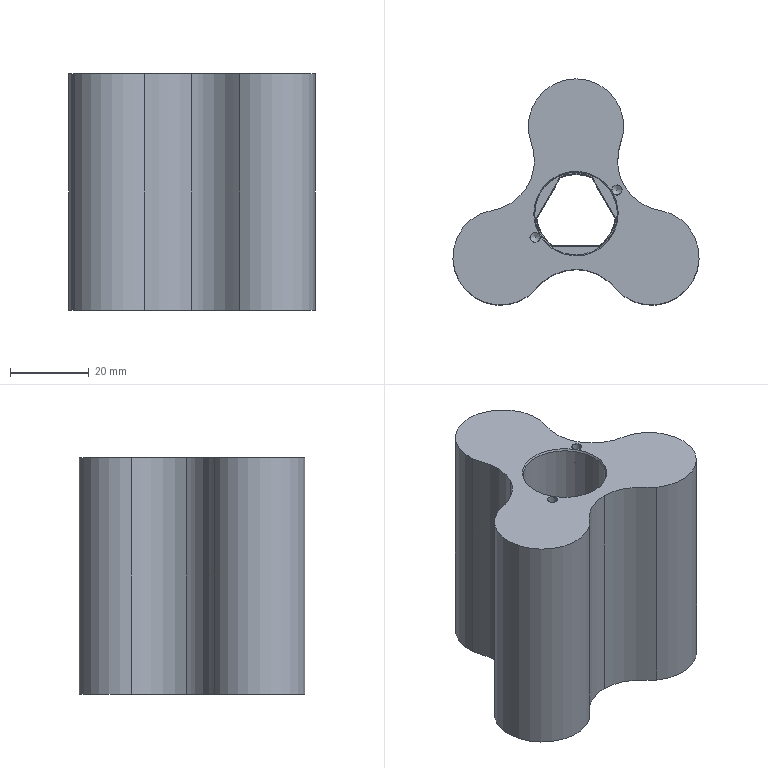Part | 1 solid | 50 faces | box 62.563 x 57.43 x 60 mm | volume 98387 mm3 | cone 18 | plane 13 | cylinder 13 | spline 6 | commonest cylinder face diameters 4.2 x3 20 x3 24.253 x3 2.5 x2 21 x1 24 x1
STEP:
#1=CARTESIAN_POINT('',(0.,-14.155,0.));
#2=VERTEX_POINT('',#1);
#3=CARTESIAN_POINT('',(-12.154,-20.96,0.));
#4=VERTEX_POINT('',#3);
#5=CARTESIAN_POINT('',(0.,-14.155,0.));
#6=CARTESIAN_POINT('',(-1.208,-14.163,0.));
#7=CARTESIAN_POINT('',(-3.582,-14.493,0.));
#8=CARTESIAN_POINT('',(-6.901,-15.987,0.));
#9=CARTESIAN_POINT('',(-9.683,-18.323,0.));
#10=CARTESIAN_POINT('',(-11.16,-20.256,0.));
#11=CARTESIAN_POINT('',(-12.154,-20.96,0.));
#12=B_SPLINE_CURVE_WITH_KNOTS('',3,(#5,#6,#7,#8,#9,#10,#11),.UNSPECIFIED.,.F.,.F.,(4,1,1,1,4),(0.,0.003576,0.007152,0.01073,0.0143),.UNSPECIFIED.);
#13=EDGE_CURVE('',#2,#4,#12,.T.);
#14=ORIENTED_EDGE('',*,*,#13,.F.);
#15=CARTESIAN_POINT('',(12.154,-20.96,0.));
#16=VERTEX_POINT('',#15);
#17=CARTESIAN_POINT('',(12.154,-20.96,0.));
#18=CARTESIAN_POINT('',(11.156,-20.253,0.));
#19=CARTESIAN_POINT('',(9.676,-18.315,0.));
#20=CARTESIAN_POINT('',(6.903,-15.991,0.));
#21=CARTESIAN_POINT('',(3.605,-14.498,0.));
#22=CARTESIAN_POINT('',(1.208,-14.163,0.));
#23=CARTESIAN_POINT('',(0.,-14.155,0.));
#24=B_SPLINE_CURVE_WITH_KNOTS('',3,(#17,#18,#19,#20,#21,#22,#23),.UNSPECIFIED.,.F.,.F.,(4,1,1,1,4),(0.,0.003619,0.007238,0.01086,0.01448),.UNSPECIFIED.);
#25=EDGE_CURVE('',#16,#2,#24,.T.);
#26=ORIENTED_EDGE('',*,*,#25,.F.);
#27=CARTESIAN_POINT('',(24.229,-0.04541,0.));
#28=VERTEX_POINT('',#27);
#29=CARTESIAN_POINT('',(19.155,-11.059,0.));
#30=DIRECTION('',(0.,0.,-1.));
#31=DIRECTION('',(-0.866,-0.5,0.));
#32=AXIS2_PLACEMENT_3D('',#29,#30,#31);
#33=CIRCLE('',#32,12.126);
#34=EDGE_CURVE('',#28,#16,#33,.T.);
#35=ORIENTED_EDGE('',*,*,#34,.F.);
#36=CARTESIAN_POINT('',(12.259,7.078,0.));
#37=VERTEX_POINT('',#36);
#38=CARTESIAN_POINT('',(12.259,7.078,0.));
#39=CARTESIAN_POINT('',(12.87,6.035,0.));
#40=CARTESIAN_POINT('',(14.342,4.144,0.));
#41=CARTESIAN_POINT('',(17.296,2.017,0.));
#42=CARTESIAN_POINT('',(20.71,0.7759,0.));
#43=CARTESIAN_POINT('',(23.122,0.4633,0.));
#44=CARTESIAN_POINT('',(24.229,-0.04541,0.));
#45=B_SPLINE_CURVE_WITH_KNOTS('',3,(#38,#39,#40,#41,#42,#43,#44),.UNSPECIFIED.,.F.,.F.,(4,1,1,1,4),(0.,0.003576,0.007152,0.01073,0.0143),.UNSPECIFIED.);
#46=EDGE_CURVE('',#37,#28,#45,.T.);
#47=ORIENTED_EDGE('',*,*,#46,.F.);
#48=CARTESIAN_POINT('',(12.075,21.006,0.));
#49=VERTEX_POINT('',#48);
#50=CARTESIAN_POINT('',(12.075,21.006,0.));
#51=CARTESIAN_POINT('',(11.962,19.788,0.));
#52=CARTESIAN_POINT('',(11.023,17.537,0.));
#53=CARTESIAN_POINT('',(10.398,13.974,0.));
#54=CARTESIAN_POINT('',(10.753,10.371,0.));
#55=CARTESIAN_POINT('',(11.662,8.128,0.));
#56=CARTESIAN_POINT('',(12.259,7.078,0.));
#57=B_SPLINE_CURVE_WITH_KNOTS('',3,(#50,#51,#52,#53,#54,#55,#56),.UNSPECIFIED.,.F.,.F.,(4,1,1,1,4),(0.,0.003619,0.007238,0.01086,0.01448),.UNSPECIFIED.);
#58=EDGE_CURVE('',#49,#37,#57,.T.);
#59=ORIENTED_EDGE('',*,*,#58,.F.);
#60=CARTESIAN_POINT('',(-12.075,21.006,0.));
#61=VERTEX_POINT('',#60);
#62=CARTESIAN_POINT('',(0.,22.118,0.));
#63=DIRECTION('',(0.,0.,-1.));
#64=DIRECTION('',(-0.866,-0.5,0.));
#65=AXIS2_PLACEMENT_3D('',#62,#63,#64);
#66=CIRCLE('',#65,12.126);
#67=EDGE_CURVE('',#61,#49,#66,.T.);
#68=ORIENTED_EDGE('',*,*,#67,.F.);
#69=CARTESIAN_POINT('',(-12.259,7.078,0.));
#70=VERTEX_POINT('',#69);
#71=CARTESIAN_POINT('',(-12.259,7.078,0.));
#72=CARTESIAN_POINT('',(-11.662,8.128,0.));
#73=CARTESIAN_POINT('',(-10.76,10.348,0.));
#74=CARTESIAN_POINT('',(-10.395,13.97,0.));
#75=CARTESIAN_POINT('',(-11.027,17.548,0.));
#76=CARTESIAN_POINT('',(-11.962,19.793,0.));
#77=CARTESIAN_POINT('',(-12.075,21.006,0.));
#78=B_SPLINE_CURVE_WITH_KNOTS('',3,(#71,#72,#73,#74,#75,#76,#77),.UNSPECIFIED.,.F.,.F.,(4,1,1,1,4),(0.,0.003576,0.007152,0.01073,0.0143),.UNSPECIFIED.);
#79=EDGE_CURVE('',#70,#61,#78,.T.);
#80=ORIENTED_EDGE('',*,*,#79,.F.);
#81=CARTESIAN_POINT('',(-24.229,-0.04543,0.));
#82=VERTEX_POINT('',#81);
#83=CARTESIAN_POINT('',(-24.229,-0.04543,0.));
#84=CARTESIAN_POINT('',(-23.118,0.4655,0.));
#85=CARTESIAN_POINT('',(-20.699,0.7776,0.));
#86=CARTESIAN_POINT('',(-17.3,2.018,0.));
#87=CARTESIAN_POINT('',(-14.358,4.127,0.));
#88=CARTESIAN_POINT('',(-12.87,6.036,0.));
#89=CARTESIAN_POINT('',(-12.259,7.078,0.));
#90=B_SPLINE_CURVE_WITH_KNOTS('',3,(#83,#84,#85,#86,#87,#88,#89),.UNSPECIFIED.,.F.,.F.,(4,1,1,1,4),(0.,0.003619,0.007238,0.01086,0.01448),.UNSPECIFIED.);
#91=EDGE_CURVE('',#82,#70,#90,.T.);
#92=ORIENTED_EDGE('',*,*,#91,.F.);
#93=CARTESIAN_POINT('',(-19.155,-11.059,0.));
#94=DIRECTION('',(0.,0.,-1.));
#95=DIRECTION('',(-0.866,-0.5,0.));
#96=AXIS2_PLACEMENT_3D('',#93,#94,#95);
#97=CIRCLE('',#96,12.126);
#98=EDGE_CURVE('',#4,#82,#97,.T.);
#99=ORIENTED_EDGE('',*,*,#98,.F.);
#100=EDGE_LOOP('',(#14,#26,#35,#47,#59,#68,#80,#92,#99));
#101=FACE_BOUND('',#100,.T.);
#102=CARTESIAN_POINT('',(-9.43,-5.126,0.));
#103=VERTEX_POINT('',#102);
#104=CARTESIAN_POINT('',(-9.154,-5.604,0.));
#105=VERTEX_POINT('',#104);
#106=CARTESIAN_POINT('',(-10.392,-6.,0.));
#107=DIRECTION('',(0.,0.,1.));
#108=DIRECTION('',(0.866,0.5,0.));
#109=AXIS2_PLACEMENT_3D('',#106,#107,#108);
#110=CIRCLE('',#109,1.3);
#111=EDGE_CURVE('',#103,#105,#110,.T.);
#112=ORIENTED_EDGE('',*,*,#111,.F.);
#113=CARTESIAN_POINT('',(9.154,5.604,0.));
#114=VERTEX_POINT('',#113);
#115=CARTESIAN_POINT('',(0.,0.,0.));
#116=DIRECTION('',(0.,0.,-1.));
#117=DIRECTION('',(-0.866,-0.5,0.));
#118=AXIS2_PLACEMENT_3D('',#115,#116,#117);
#119=CIRCLE('',#118,10.733);
#120=EDGE_CURVE('',#103,#114,#119,.T.);
#121=ORIENTED_EDGE('',*,*,#120,.T.);
#122=CARTESIAN_POINT('',(9.43,5.126,0.));
#123=VERTEX_POINT('',#122);
#124=CARTESIAN_POINT('',(10.392,6.,0.));
#125=DIRECTION('',(0.,0.,1.));
#126=DIRECTION('',(0.866,0.5,0.));
#127=AXIS2_PLACEMENT_3D('',#124,#125,#126);
#128=CIRCLE('',#127,1.3);
#129=EDGE_CURVE('',#123,#114,#128,.T.);
#130=ORIENTED_EDGE('',*,*,#129,.F.);
#131=CARTESIAN_POINT('',(0.,0.,0.));
#132=DIRECTION('',(0.,0.,-1.));
#133=DIRECTION('',(-0.866,-0.5,0.));
#134=AXIS2_PLACEMENT_3D('',#131,#132,#133);
#135=CIRCLE('',#134,10.733);
#136=EDGE_CURVE('',#123,#105,#135,.T.);
#137=ORIENTED_EDGE('',*,*,#136,.T.);
#138=EDGE_LOOP('',(#112,#121,#130,#137));
#139=FACE_BOUND('',#138,.T.);
#140=CARTESIAN_POINT('',(-6.815,-16.188,0.));
#141=DIRECTION('',(0.,0.,-1.));
#142=DIRECTION('',(-0.866,-0.5,0.));
#143=AXIS2_PLACEMENT_3D('',#140,#141,#142);
#144=PLANE('',#143);
#145=ADVANCED_FACE('',(#101,#139),#144,.F.);
#146=CARTESIAN_POINT('',(3.928,9.196,-50.3));
#147=VERTEX_POINT('',#146);
#148=CARTESIAN_POINT('',(3.928,9.196,-15.4));
#149=VERTEX_POINT('',#148);
#150=CARTESIAN_POINT('',(3.928,9.196,-60.));
#151=DIRECTION('',(0.,0.,1.));
#152=VECTOR('',#151,1000.);
#153=LINE('',#150,#152);
#154=EDGE_CURVE('',#147,#149,#153,.T.);
#155=ORIENTED_EDGE('',*,*,#154,.T.);
#156=CARTESIAN_POINT('',(-3.928,9.196,-15.4));
#157=VERTEX_POINT('',#156);
#158=CARTESIAN_POINT('',(0.,0.,-15.4));
#159=DIRECTION('',(0.,0.,1.));
#160=DIRECTION('',(0.866,0.5,0.));
#161=AXIS2_PLACEMENT_3D('',#158,#159,#160);
#162=CIRCLE('',#161,10.);
#163=EDGE_CURVE('',#149,#157,#162,.T.);
#164=ORIENTED_EDGE('',*,*,#163,.T.);
#165=CARTESIAN_POINT('',(-3.928,9.196,-50.3));
#166=VERTEX_POINT('',#165);
#167=CARTESIAN_POINT('',(-3.928,9.196,-60.));
#168=DIRECTION('',(0.,0.,1.));
#169=VECTOR('',#168,1000.);
#170=LINE('',#167,#169);
#171=EDGE_CURVE('',#166,#157,#170,.T.);
#172=ORIENTED_EDGE('',*,*,#171,.F.);
#173=CARTESIAN_POINT('',(0.,0.,-50.3));
#174=DIRECTION('',(0.,0.,-1.));
#175=DIRECTION('',(-0.866,-0.5,0.));
#176=AXIS2_PLACEMENT_3D('',#173,#174,#175);
#177=CIRCLE('',#176,10.);
#178=EDGE_CURVE('',#166,#147,#177,.T.);
#179=ORIENTED_EDGE('',*,*,#178,.T.);
#180=EDGE_LOOP('',(#155,#164,#172,#179));
#181=FACE_BOUND('',#180,.T.);
#182=CARTESIAN_POINT('',(0.,0.,-60.));
#183=DIRECTION('',(0.,0.,1.));
#184=DIRECTION('',(0.866,0.5,0.));
#185=AXIS2_PLACEMENT_3D('',#182,#183,#184);
#186=CYLINDRICAL_SURFACE('',#185,10.);
#187=ADVANCED_FACE('',(#181),#186,.F.);
#188=CARTESIAN_POINT('',(9.928,-1.196,-50.3));
#189=VERTEX_POINT('',#188);
#190=CARTESIAN_POINT('',(9.928,-1.196,-15.4));
#191=VERTEX_POINT('',#190);
#192=CARTESIAN_POINT('',(9.928,-1.196,-60.));
#193=DIRECTION('',(0.,0.,1.));
#194=VECTOR('',#193,1000.);
#195=LINE('',#192,#194);
#196=EDGE_CURVE('',#189,#191,#195,.T.);
#197=ORIENTED_EDGE('',*,*,#196,.T.);
#198=CARTESIAN_POINT('',(3.928,9.196,-15.4));
#199=DIRECTION('',(-0.5,0.866,0.));
#200=VECTOR('',#199,1000.);
#201=LINE('',#198,#200);
#202=EDGE_CURVE('',#191,#149,#201,.T.);
#203=ORIENTED_EDGE('',*,*,#202,.T.);
#204=ORIENTED_EDGE('',*,*,#154,.F.);
#205=CARTESIAN_POINT('',(9.928,-1.196,-50.3));
#206=DIRECTION('',(0.5,-0.866,0.));
#207=VECTOR('',#206,1000.);
#208=LINE('',#205,#207);
#209=EDGE_CURVE('',#147,#189,#208,.T.);
#210=ORIENTED_EDGE('',*,*,#209,.T.);
#211=EDGE_LOOP('',(#197,#203,#204,#210));
#212=FACE_BOUND('',#211,.T.);
#213=CARTESIAN_POINT('',(3.928,9.196,-60.));
#214=DIRECTION('',(0.866,0.5,0.));
#215=DIRECTION('',(0.,0.,-1.));
#216=AXIS2_PLACEMENT_3D('',#213,#214,#215);
#217=PLANE('',#216);
#218=ADVANCED_FACE('',(#212),#217,.F.);
#219=CARTESIAN_POINT('',(6.,-8.,-50.3));
#220=VERTEX_POINT('',#219);
#221=CARTESIAN_POINT('',(6.,-8.,-15.4));
#222=VERTEX_POINT('',#221);
#223=CARTESIAN_POINT('',(6.,-8.,-60.));
#224=DIRECTION('',(0.,0.,1.));
#225=VECTOR('',#224,1000.);
#226=LINE('',#223,#225);
#227=EDGE_CURVE('',#220,#222,#226,.T.);
#228=ORIENTED_EDGE('',*,*,#227,.T.);
#229=CARTESIAN_POINT('',(0.,0.,-15.4));
#230=DIRECTION('',(0.,0.,1.));
#231=DIRECTION('',(0.866,0.5,0.));
#232=AXIS2_PLACEMENT_3D('',#229,#230,#231);
#233=CIRCLE('',#232,10.);
#234=EDGE_CURVE('',#222,#191,#233,.T.);
#235=ORIENTED_EDGE('',*,*,#234,.T.);
#236=ORIENTED_EDGE('',*,*,#196,.F.);
#237=CARTESIAN_POINT('',(0.,0.,-50.3));
#238=DIRECTION('',(0.,0.,-1.));
#239=DIRECTION('',(-0.866,-0.5,0.));
#240=AXIS2_PLACEMENT_3D('',#237,#238,#239);
#241=CIRCLE('',#240,10.);
#242=EDGE_CURVE('',#189,#220,#241,.T.);
#243=ORIENTED_EDGE('',*,*,#242,.T.);
#244=EDGE_LOOP('',(#228,#235,#236,#243));
#245=FACE_BOUND('',#244,.T.);
#246=CARTESIAN_POINT('',(0.,0.,-60.));
#247=DIRECTION('',(0.,0.,1.));
#248=DIRECTION('',(0.866,0.5,0.));
#249=AXIS2_PLACEMENT_3D('',#246,#247,#248);
#250=CYLINDRICAL_SURFACE('',#249,10.);
#251=ADVANCED_FACE('',(#245),#250,.F.);
#252=CARTESIAN_POINT('',(-6.,-8.,-50.3));
#253=VERTEX_POINT('',#252);
#254=CARTESIAN_POINT('',(-6.,-8.,-15.4));
#255=VERTEX_POINT('',#254);
#256=CARTESIAN_POINT('',(-6.,-8.,-60.));
#257=DIRECTION('',(0.,0.,1.));
#258=VECTOR('',#257,1000.);
#259=LINE('',#256,#258);
#260=EDGE_CURVE('',#253,#255,#259,.T.);
#261=ORIENTED_EDGE('',*,*,#260,.T.);
#262=CARTESIAN_POINT('',(6.,-8.,-15.4));
#263=DIRECTION('',(1.,0.,0.));
#264=VECTOR('',#263,1000.);
#265=LINE('',#262,#264);
#266=EDGE_CURVE('',#255,#222,#265,.T.);
#267=ORIENTED_EDGE('',*,*,#266,.T.);
#268=ORIENTED_EDGE('',*,*,#227,.F.);
#269=CARTESIAN_POINT('',(-6.,-8.,-50.3));
#270=DIRECTION('',(-1.,0.,0.));
#271=VECTOR('',#270,1000.);
#272=LINE('',#269,#271);
#273=EDGE_CURVE('',#220,#253,#272,.T.);
#274=ORIENTED_EDGE('',*,*,#273,.T.);
#275=EDGE_LOOP('',(#261,#267,#268,#274));
#276=FACE_BOUND('',#275,.T.);
#277=CARTESIAN_POINT('',(6.,-8.,-60.));
#278=DIRECTION('',(0.,-1.,0.));
#279=DIRECTION('',(-1.,0.,0.));
#280=AXIS2_PLACEMENT_3D('',#277,#278,#279);
#281=PLANE('',#280);
#282=ADVANCED_FACE('',(#276),#281,.F.);
#283=CARTESIAN_POINT('',(-9.928,-1.196,-50.3));
#284=VERTEX_POINT('',#283);
#285=CARTESIAN_POINT('',(-9.928,-1.196,-15.4));
#286=VERTEX_POINT('',#285);
#287=CARTESIAN_POINT('',(-9.928,-1.196,-60.));
#288=DIRECTION('',(0.,0.,1.));
#289=VECTOR('',#288,1000.);
#290=LINE('',#287,#289);
#291=EDGE_CURVE('',#284,#286,#290,.T.);
#292=ORIENTED_EDGE('',*,*,#291,.T.);
#293=CARTESIAN_POINT('',(0.,0.,-15.4));
#294=DIRECTION('',(0.,0.,1.));
#295=DIRECTION('',(0.866,0.5,0.));
#296=AXIS2_PLACEMENT_3D('',#293,#294,#295);
#297=CIRCLE('',#296,10.);
#298=EDGE_CURVE('',#286,#255,#297,.T.);
#299=ORIENTED_EDGE('',*,*,#298,.T.);
#300=ORIENTED_EDGE('',*,*,#260,.F.);
#301=CARTESIAN_POINT('',(0.,0.,-50.3));
#302=DIRECTION('',(0.,0.,-1.));
#303=DIRECTION('',(-0.866,-0.5,0.));
#304=AXIS2_PLACEMENT_3D('',#301,#302,#303);
#305=CIRCLE('',#304,10.);
#306=EDGE_CURVE('',#253,#284,#305,.T.);
#307=ORIENTED_EDGE('',*,*,#306,.T.);
#308=EDGE_LOOP('',(#292,#299,#300,#307));
#309=FACE_BOUND('',#308,.T.);
#310=CARTESIAN_POINT('',(0.,0.,-60.));
#311=DIRECTION('',(0.,0.,1.));
#312=DIRECTION('',(0.866,0.5,0.));
#313=AXIS2_PLACEMENT_3D('',#310,#311,#312);
#314=CYLINDRICAL_SURFACE('',#313,10.);
#315=ADVANCED_FACE('',(#309),#314,.F.);
#316=ORIENTED_EDGE('',*,*,#171,.T.);
#317=CARTESIAN_POINT('',(-9.928,-1.196,-15.4));
#318=DIRECTION('',(-0.5,-0.866,0.));
#319=VECTOR('',#318,1000.);
#320=LINE('',#317,#319);
#321=EDGE_CURVE('',#157,#286,#320,.T.);
#322=ORIENTED_EDGE('',*,*,#321,.T.);
#323=ORIENTED_EDGE('',*,*,#291,.F.);
#324=CARTESIAN_POINT('',(-3.928,9.196,-50.3));
#325=DIRECTION('',(0.5,0.866,0.));
#326=VECTOR('',#325,1000.);
#327=LINE('',#324,#326);
#328=EDGE_CURVE('',#284,#166,#327,.T.);
#329=ORIENTED_EDGE('',*,*,#328,.T.);
#330=EDGE_LOOP('',(#316,#322,#323,#329));
#331=FACE_BOUND('',#330,.T.);
#332=CARTESIAN_POINT('',(-9.928,-1.196,-60.));
#333=DIRECTION('',(-0.866,0.5,0.));
#334=DIRECTION('',(0.5,0.866,0.));
#335=AXIS2_PLACEMENT_3D('',#332,#333,#334);
#336=PLANE('',#335);
#337=ADVANCED_FACE('',(#331),#336,.F.);
#338=ORIENTED_EDGE('',*,*,#13,.T.);
#339=CARTESIAN_POINT('',(-12.154,-20.96,-60.));
#340=VERTEX_POINT('',#339);
#341=CARTESIAN_POINT('',(-12.154,-20.96,-60.));
#342=DIRECTION('',(0.,0.,1.));
#343=VECTOR('',#342,1000.);
#344=LINE('',#341,#343);
#345=EDGE_CURVE('',#340,#4,#344,.T.);
#346=ORIENTED_EDGE('',*,*,#345,.F.);
#347=CARTESIAN_POINT('',(0.,-14.155,-60.));
#348=VERTEX_POINT('',#347);
#349=CARTESIAN_POINT('',(0.,-14.155,-60.));
#350=CARTESIAN_POINT('',(-1.208,-14.163,-60.));
#351=CARTESIAN_POINT('',(-3.582,-14.493,-60.));
#352=CARTESIAN_POINT('',(-6.901,-15.987,-60.));
#353=CARTESIAN_POINT('',(-9.683,-18.323,-60.));
#354=CARTESIAN_POINT('',(-11.16,-20.256,-60.));
#355=CARTESIAN_POINT('',(-12.154,-20.96,-60.));
#356=B_SPLINE_CURVE_WITH_KNOTS('',3,(#349,#350,#351,#352,#353,#354,#355),.UNSPECIFIED.,.F.,.F.,(4,1,1,1,4),(0.,0.003576,0.007152,0.01073,0.0143),.UNSPECIFIED.);
#357=EDGE_CURVE('',#348,#340,#356,.T.);
#358=ORIENTED_EDGE('',*,*,#357,.F.);
#359=CARTESIAN_POINT('',(0.,-14.155,-60.));
#360=DIRECTION('',(0.,0.,1.));
#361=VECTOR('',#360,1000.);
#362=LINE('',#359,#361);
#363=EDGE_CURVE('',#348,#2,#362,.T.);
#364=ORIENTED_EDGE('',*,*,#363,.T.);
#365=EDGE_LOOP('',(#338,#346,#358,#364));
#366=FACE_BOUND('',#365,.T.);
#367=CARTESIAN_POINT('',(0.,-14.155,-60.));
#368=CARTESIAN_POINT('',(0.,-14.155,0.));
#369=CARTESIAN_POINT('',(-1.199,-14.163,-60.));
#370=CARTESIAN_POINT('',(-1.199,-14.163,0.));
#371=CARTESIAN_POINT('',(-3.611,-14.497,-60.));
#372=CARTESIAN_POINT('',(-3.611,-14.497,0.));
#373=CARTESIAN_POINT('',(-6.932,-16.006,-60.));
#374=CARTESIAN_POINT('',(-6.932,-16.006,0.));
#375=CARTESIAN_POINT('',(-9.709,-18.356,-60.));
#376=CARTESIAN_POINT('',(-9.709,-18.356,0.));
#377=CARTESIAN_POINT('',(-11.176,-20.267,-60.));
#378=CARTESIAN_POINT('',(-11.176,-20.267,0.));
#379=CARTESIAN_POINT('',(-12.154,-20.96,-60.));
#380=CARTESIAN_POINT('',(-12.154,-20.96,0.));
#381=B_SPLINE_SURFACE_WITH_KNOTS('',3,1,((#367,#368),(#369,#370),(#371,#372),(#373,#374),(#375,#376),(#377,#378),(#379,#380)),.SURF_OF_LINEAR_EXTRUSION.,.F.,.F.,.F.,(4,1,1,1,4),(2,2),(-0.00002345,0.25,0.5,0.75,1.),(0.,1.),.UNSPECIFIED.);
#382=ADVANCED_FACE('',(#366),#381,.F.);
#383=ORIENTED_EDGE('',*,*,#98,.T.);
#384=CARTESIAN_POINT('',(-24.229,-0.04543,-60.));
#385=VERTEX_POINT('',#384);
#386=CARTESIAN_POINT('',(-24.229,-0.04543,-60.));
#387=DIRECTION('',(0.,0.,1.));
#388=VECTOR('',#387,1000.);
#389=LINE('',#386,#388);
#390=EDGE_CURVE('',#385,#82,#389,.T.);
#391=ORIENTED_EDGE('',*,*,#390,.F.);
#392=CARTESIAN_POINT('',(-19.155,-11.059,-60.));
#393=DIRECTION('',(0.,0.,-1.));
#394=DIRECTION('',(-0.866,-0.5,0.));
#395=AXIS2_PLACEMENT_3D('',#392,#393,#394);
#396=CIRCLE('',#395,12.126);
#397=EDGE_CURVE('',#340,#385,#396,.T.);
#398=ORIENTED_EDGE('',*,*,#397,.F.);
#399=ORIENTED_EDGE('',*,*,#345,.T.);
#400=EDGE_LOOP('',(#383,#391,#398,#399));
#401=FACE_BOUND('',#400,.T.);
#402=CARTESIAN_POINT('',(-19.155,-11.059,-60.));
#403=DIRECTION('',(0.,0.,1.));
#404=DIRECTION('',(0.866,0.5,0.));
#405=AXIS2_PLACEMENT_3D('',#402,#403,#404);
#406=CYLINDRICAL_SURFACE('',#405,12.126);
#407=ADVANCED_FACE('',(#401),#406,.T.);
#408=ORIENTED_EDGE('',*,*,#91,.T.);
#409=CARTESIAN_POINT('',(-12.259,7.078,-60.));
#410=VERTEX_POINT('',#409);
#411=CARTESIAN_POINT('',(-12.259,7.078,-60.));
#412=DIRECTION('',(0.,0.,1.));
#413=VECTOR('',#412,1000.);
#414=LINE('',#411,#413);
#415=EDGE_CURVE('',#410,#70,#414,.T.);
#416=ORIENTED_EDGE('',*,*,#415,.F.);
#417=CARTESIAN_POINT('',(-24.229,-0.04543,-60.));
#418=CARTESIAN_POINT('',(-23.118,0.4655,-60.));
#419=CARTESIAN_POINT('',(-20.699,0.7776,-60.));
#420=CARTESIAN_POINT('',(-17.3,2.018,-60.));
#421=CARTESIAN_POINT('',(-14.358,4.127,-60.));
#422=CARTESIAN_POINT('',(-12.87,6.036,-60.));
#423=CARTESIAN_POINT('',(-12.259,7.078,-60.));
#424=B_SPLINE_CURVE_WITH_KNOTS('',3,(#417,#418,#419,#420,#421,#422,#423),.UNSPECIFIED.,.F.,.F.,(4,1,1,1,4),(0.,0.003619,0.007238,0.01086,0.01448),.UNSPECIFIED.);
#425=EDGE_CURVE('',#385,#410,#424,.T.);
#426=ORIENTED_EDGE('',*,*,#425,.F.);
#427=ORIENTED_EDGE('',*,*,#390,.T.);
#428=EDGE_LOOP('',(#408,#416,#426,#427));
#429=FACE_BOUND('',#428,.T.);
#430=CARTESIAN_POINT('',(-24.229,-0.04543,-60.));
#431=CARTESIAN_POINT('',(-24.229,-0.04543,0.));
#432=CARTESIAN_POINT('',(-23.14,0.4552,-60.));
#433=CARTESIAN_POINT('',(-23.14,0.4552,0.));
#434=CARTESIAN_POINT('',(-20.752,0.7702,-60.));
#435=CARTESIAN_POINT('',(-20.752,0.7702,0.));
#436=CARTESIAN_POINT('',(-17.327,2.,-60.));
#437=CARTESIAN_POINT('',(-17.327,2.,0.));
#438=CARTESIAN_POINT('',(-14.361,4.121,-60.));
#439=CARTESIAN_POINT('',(-14.361,4.121,0.));
#440=CARTESIAN_POINT('',(-12.865,6.044,-60.));
#441=CARTESIAN_POINT('',(-12.865,6.044,0.));
#442=CARTESIAN_POINT('',(-12.259,7.078,-60.));
#443=CARTESIAN_POINT('',(-12.259,7.078,0.));
#444=B_SPLINE_SURFACE_WITH_KNOTS('',3,1,((#430,#431),(#432,#433),(#434,#435),(#436,#437),(#438,#439),(#440,#441),(#442,#443)),.SURF_OF_LINEAR_EXTRUSION.,.F.,.F.,.F.,(4,1,1,1,4),(2,2),(0.,0.25,0.5,0.75,1.),(0.,1.),.UNSPECIFIED.);
#445=ADVANCED_FACE('',(#429),#444,.F.);
#446=ORIENTED_EDGE('',*,*,#79,.T.);
#447=CARTESIAN_POINT('',(-12.075,21.006,-60.));
#448=VERTEX_POINT('',#447);
#449=CARTESIAN_POINT('',(-12.075,21.006,-60.));
#450=DIRECTION('',(0.,0.,1.));
#451=VECTOR('',#450,1000.);
#452=LINE('',#449,#451);
#453=EDGE_CURVE('',#448,#61,#452,.T.);
#454=ORIENTED_EDGE('',*,*,#453,.F.);
#455=CARTESIAN_POINT('',(-12.259,7.078,-60.));
#456=CARTESIAN_POINT('',(-11.662,8.128,-60.));
#457=CARTESIAN_POINT('',(-10.76,10.348,-60.));
#458=CARTESIAN_POINT('',(-10.395,13.97,-60.));
#459=CARTESIAN_POINT('',(-11.027,17.548,-60.));
#460=CARTESIAN_POINT('',(-11.962,19.793,-60.));
#461=CARTESIAN_POINT('',(-12.075,21.006,-60.));
#462=B_SPLINE_CURVE_WITH_KNOTS('',3,(#455,#456,#457,#458,#459,#460,#461),.UNSPECIFIED.,.F.,.F.,(4,1,1,1,4),(0.,0.003576,0.007152,0.01073,0.0143),.UNSPECIFIED.);
#463=EDGE_CURVE('',#410,#448,#462,.T.);
#464=ORIENTED_EDGE('',*,*,#463,.F.);
#465=ORIENTED_EDGE('',*,*,#415,.T.);
#466=EDGE_LOOP('',(#446,#454,#464,#465));
#467=FACE_BOUND('',#466,.T.);
#468=CARTESIAN_POINT('',(-12.259,7.078,-60.));
#469=CARTESIAN_POINT('',(-12.259,7.078,0.));
#470=CARTESIAN_POINT('',(-11.666,8.12,-60.));
#471=CARTESIAN_POINT('',(-11.666,8.12,0.));
#472=CARTESIAN_POINT('',(-10.749,10.376,-60.));
#473=CARTESIAN_POINT('',(-10.749,10.376,0.));
#474=CARTESIAN_POINT('',(-10.395,14.006,-60.));
#475=CARTESIAN_POINT('',(-10.395,14.006,0.));
#476=CARTESIAN_POINT('',(-11.043,17.586,-60.));
#477=CARTESIAN_POINT('',(-11.043,17.586,0.));
#478=CARTESIAN_POINT('',(-11.964,19.812,-60.));
#479=CARTESIAN_POINT('',(-11.964,19.812,0.));
#480=CARTESIAN_POINT('',(-12.075,21.006,-60.));
#481=CARTESIAN_POINT('',(-12.075,21.006,0.));
#482=B_SPLINE_SURFACE_WITH_KNOTS('',3,1,((#468,#469),(#470,#471),(#472,#473),(#474,#475),(#476,#477),(#478,#479),(#480,#481)),.SURF_OF_LINEAR_EXTRUSION.,.F.,.F.,.F.,(4,1,1,1,4),(2,2),(-0.00002345,0.25,0.5,0.75,1.),(0.,1.),.UNSPECIFIED.);
#483=ADVANCED_FACE('',(#467),#482,.F.);
#484=ORIENTED_EDGE('',*,*,#67,.T.);
#485=CARTESIAN_POINT('',(12.075,21.006,-60.));
#486=VERTEX_POINT('',#485);
#487=CARTESIAN_POINT('',(12.075,21.006,-60.));
#488=DIRECTION('',(0.,0.,1.));
#489=VECTOR('',#488,1000.);
#490=LINE('',#487,#489);
#491=EDGE_CURVE('',#486,#49,#490,.T.);
#492=ORIENTED_EDGE('',*,*,#491,.F.);
#493=CARTESIAN_POINT('',(0.,22.118,-60.));
#494=DIRECTION('',(0.,0.,-1.));
#495=DIRECTION('',(-0.866,-0.5,0.));
#496=AXIS2_PLACEMENT_3D('',#493,#494,#495);
#497=CIRCLE('',#496,12.126);
#498=EDGE_CURVE('',#448,#486,#497,.T.);
#499=ORIENTED_EDGE('',*,*,#498,.F.);
#500=ORIENTED_EDGE('',*,*,#453,.T.);
#501=EDGE_LOOP('',(#484,#492,#499,#500));
#502=FACE_BOUND('',#501,.T.);
#503=CARTESIAN_POINT('',(0.,22.118,-60.));
#504=DIRECTION('',(0.,0.,1.));
#505=DIRECTION('',(0.866,0.5,0.));
#506=AXIS2_PLACEMENT_3D('',#503,#504,#505);
#507=CYLINDRICAL_SURFACE('',#506,12.126);
#508=ADVANCED_FACE('',(#502),#507,.T.);
#509=ORIENTED_EDGE('',*,*,#58,.T.);
#510=CARTESIAN_POINT('',(12.259,7.078,-60.));
#511=VERTEX_POINT('',#510);
#512=CARTESIAN_POINT('',(12.259,7.078,-60.));
#513=DIRECTION('',(0.,0.,1.));
#514=VECTOR('',#513,1000.);
#515=LINE('',#512,#514);
#516=EDGE_CURVE('',#511,#37,#515,.T.);
#517=ORIENTED_EDGE('',*,*,#516,.F.);
#518=CARTESIAN_POINT('',(12.075,21.006,-60.));
#519=CARTESIAN_POINT('',(11.962,19.788,-60.));
#520=CARTESIAN_POINT('',(11.023,17.537,-60.));
#521=CARTESIAN_POINT('',(10.398,13.974,-60.));
#522=CARTESIAN_POINT('',(10.753,10.371,-60.));
#523=CARTESIAN_POINT('',(11.662,8.128,-60.));
#524=CARTESIAN_POINT('',(12.259,7.078,-60.));
#525=B_SPLINE_CURVE_WITH_KNOTS('',3,(#518,#519,#520,#521,#522,#523,#524),.UNSPECIFIED.,.F.,.F.,(4,1,1,1,4),(0.,0.003619,0.007238,0.01086,0.01448),.UNSPECIFIED.);
#526=EDGE_CURVE('',#486,#511,#525,.T.);
#527=ORIENTED_EDGE('',*,*,#526,.F.);
#528=ORIENTED_EDGE('',*,*,#491,.T.);
#529=EDGE_LOOP('',(#509,#517,#527,#528));
#530=FACE_BOUND('',#529,.T.);
#531=CARTESIAN_POINT('',(12.075,21.006,-60.));
#532=CARTESIAN_POINT('',(12.075,21.006,0.));
#533=CARTESIAN_POINT('',(11.964,19.812,-60.));
#534=CARTESIAN_POINT('',(11.964,19.812,0.));
#535=CARTESIAN_POINT('',(11.043,17.586,-60.));
#536=CARTESIAN_POINT('',(11.043,17.586,0.));
#537=CARTESIAN_POINT('',(10.395,14.006,-60.));
#538=CARTESIAN_POINT('',(10.395,14.006,0.));
#539=CARTESIAN_POINT('',(10.749,10.376,-60.));
#540=CARTESIAN_POINT('',(10.749,10.376,0.));
#541=CARTESIAN_POINT('',(11.666,8.12,-60.));
#542=CARTESIAN_POINT('',(11.666,8.12,0.));
#543=CARTESIAN_POINT('',(12.259,7.078,-60.));
#544=CARTESIAN_POINT('',(12.259,7.078,0.));
#545=B_SPLINE_SURFACE_WITH_KNOTS('',3,1,((#531,#532),(#533,#534),(#535,#536),(#537,#538),(#539,#540),(#541,#542),(#543,#544)),.SURF_OF_LINEAR_EXTRUSION.,.F.,.F.,.F.,(4,1,1,1,4),(2,2),(0.,0.25,0.5,0.75,1.),(0.,1.),.UNSPECIFIED.);
#546=ADVANCED_FACE('',(#530),#545,.F.);
#547=ORIENTED_EDGE('',*,*,#46,.T.);
#548=CARTESIAN_POINT('',(24.229,-0.04541,-60.));
#549=VERTEX_POINT('',#548);
#550=CARTESIAN_POINT('',(24.229,-0.04541,-60.));
#551=DIRECTION('',(0.,0.,1.));
#552=VECTOR('',#551,1000.);
#553=LINE('',#550,#552);
#554=EDGE_CURVE('',#549,#28,#553,.T.);
#555=ORIENTED_EDGE('',*,*,#554,.F.);
#556=CARTESIAN_POINT('',(12.259,7.078,-60.));
#557=CARTESIAN_POINT('',(12.87,6.035,-60.));
#558=CARTESIAN_POINT('',(14.342,4.144,-60.));
#559=CARTESIAN_POINT('',(17.296,2.017,-60.));
#560=CARTESIAN_POINT('',(20.71,0.7759,-60.));
#561=CARTESIAN_POINT('',(23.122,0.4633,-60.));
#562=CARTESIAN_POINT('',(24.229,-0.04541,-60.));
#563=B_SPLINE_CURVE_WITH_KNOTS('',3,(#556,#557,#558,#559,#560,#561,#562),.UNSPECIFIED.,.F.,.F.,(4,1,1,1,4),(0.,0.003576,0.007152,0.01073,0.0143),.UNSPECIFIED.);
#564=EDGE_CURVE('',#511,#549,#563,.T.);
#565=ORIENTED_EDGE('',*,*,#564,.F.);
#566=ORIENTED_EDGE('',*,*,#516,.T.);
#567=EDGE_LOOP('',(#547,#555,#565,#566));
#568=FACE_BOUND('',#567,.T.);
#569=CARTESIAN_POINT('',(12.259,7.078,-60.));
#570=CARTESIAN_POINT('',(12.259,7.078,0.));
#571=CARTESIAN_POINT('',(12.865,6.044,-60.));
#572=CARTESIAN_POINT('',(12.865,6.044,0.));
#573=CARTESIAN_POINT('',(14.361,4.121,-60.));
#574=CARTESIAN_POINT('',(14.361,4.121,0.));
#575=CARTESIAN_POINT('',(17.327,2.,-60.));
#576=CARTESIAN_POINT('',(17.327,2.,0.));
#577=CARTESIAN_POINT('',(20.751,0.7702,-60.));
#578=CARTESIAN_POINT('',(20.751,0.7702,0.));
#579=CARTESIAN_POINT('',(23.14,0.4553,-60.));
#580=CARTESIAN_POINT('',(23.14,0.4553,0.));
#581=CARTESIAN_POINT('',(24.229,-0.04541,-60.));
#582=CARTESIAN_POINT('',(24.229,-0.04541,0.));
#583=B_SPLINE_SURFACE_WITH_KNOTS('',3,1,((#569,#570),(#571,#572),(#573,#574),(#575,#576),(#577,#578),(#579,#580),(#581,#582)),.SURF_OF_LINEAR_EXTRUSION.,.F.,.F.,.F.,(4,1,1,1,4),(2,2),(-0.00002345,0.25,0.5,0.75,1.),(0.,1.),.UNSPECIFIED.);
#584=ADVANCED_FACE('',(#568),#583,.F.);
#585=ORIENTED_EDGE('',*,*,#34,.T.);
#586=CARTESIAN_POINT('',(12.154,-20.96,-60.));
#587=VERTEX_POINT('',#586);
#588=CARTESIAN_POINT('',(12.154,-20.96,-60.));
#589=DIRECTION('',(0.,0.,1.));
#590=VECTOR('',#589,1000.);
#591=LINE('',#588,#590);
#592=EDGE_CURVE('',#587,#16,#591,.T.);
#593=ORIENTED_EDGE('',*,*,#592,.F.);
#594=CARTESIAN_POINT('',(19.155,-11.059,-60.));
#595=DIRECTION('',(0.,0.,-1.));
#596=DIRECTION('',(-0.866,-0.5,0.));
#597=AXIS2_PLACEMENT_3D('',#594,#595,#596);
#598=CIRCLE('',#597,12.126);
#599=EDGE_CURVE('',#549,#587,#598,.T.);
#600=ORIENTED_EDGE('',*,*,#599,.F.);
#601=ORIENTED_EDGE('',*,*,#554,.T.);
#602=EDGE_LOOP('',(#585,#593,#600,#601));
#603=FACE_BOUND('',#602,.T.);
#604=CARTESIAN_POINT('',(19.155,-11.059,-60.));
#605=DIRECTION('',(0.,0.,1.));
#606=DIRECTION('',(0.866,0.5,0.));
#607=AXIS2_PLACEMENT_3D('',#604,#605,#606);
#608=CYLINDRICAL_SURFACE('',#607,12.126);
#609=ADVANCED_FACE('',(#603),#608,.T.);
#610=ORIENTED_EDGE('',*,*,#25,.T.);
#611=ORIENTED_EDGE('',*,*,#363,.F.);
#612=CARTESIAN_POINT('',(12.154,-20.96,-60.));
#613=CARTESIAN_POINT('',(11.156,-20.253,-60.));
#614=CARTESIAN_POINT('',(9.676,-18.315,-60.));
#615=CARTESIAN_POINT('',(6.903,-15.991,-60.));
#616=CARTESIAN_POINT('',(3.605,-14.498,-60.));
#617=CARTESIAN_POINT('',(1.208,-14.163,-60.));
#618=CARTESIAN_POINT('',(0.,-14.155,-60.));
#619=B_SPLINE_CURVE_WITH_KNOTS('',3,(#612,#613,#614,#615,#616,#617,#618),.UNSPECIFIED.,.F.,.F.,(4,1,1,1,4),(0.,0.003619,0.007238,0.01086,0.01448),.UNSPECIFIED.);
#620=EDGE_CURVE('',#587,#348,#619,.T.);
#621=ORIENTED_EDGE('',*,*,#620,.F.);
#622=ORIENTED_EDGE('',*,*,#592,.T.);
#623=EDGE_LOOP('',(#610,#611,#621,#622));
#624=FACE_BOUND('',#623,.T.);
#625=CARTESIAN_POINT('',(12.154,-20.96,-60.));
#626=CARTESIAN_POINT('',(12.154,-20.96,0.));
#627=CARTESIAN_POINT('',(11.176,-20.267,-60.));
#628=CARTESIAN_POINT('',(11.176,-20.267,0.));
#629=CARTESIAN_POINT('',(9.709,-18.356,-60.));
#630=CARTESIAN_POINT('',(9.709,-18.356,0.));
#631=CARTESIAN_POINT('',(6.932,-16.006,-60.));
#632=CARTESIAN_POINT('',(6.932,-16.006,0.));
#633=CARTESIAN_POINT('',(3.611,-14.497,-60.));
#634=CARTESIAN_POINT('',(3.611,-14.497,0.));
#635=CARTESIAN_POINT('',(1.199,-14.163,-60.));
#636=CARTESIAN_POINT('',(1.199,-14.163,0.));
#637=CARTESIAN_POINT('',(0.,-14.155,-60.));
#638=CARTESIAN_POINT('',(0.,-14.155,0.));
#639=B_SPLINE_SURFACE_WITH_KNOTS('',3,1,((#625,#626),(#627,#628),(#629,#630),(#631,#632),(#633,#634),(#635,#636),(#637,#638)),.SURF_OF_LINEAR_EXTRUSION.,.F.,.F.,.F.,(4,1,1,1,4),(2,2),(0.,0.25,0.5,0.75,1.),(0.,1.),.UNSPECIFIED.);
#640=ADVANCED_FACE('',(#624),#639,.F.);
#641=CARTESIAN_POINT('',(-10.566,-6.1,-60.));
#642=VERTEX_POINT('',#641);
#643=CARTESIAN_POINT('',(0.,0.,-60.));
#644=DIRECTION('',(0.,0.,-1.));
#645=DIRECTION('',(-0.866,-0.5,0.));
#646=AXIS2_PLACEMENT_3D('',#643,#644,#645);
#647=CIRCLE('',#646,12.2);
#648=EDGE_CURVE('',#642,#642,#647,.F.);
#649=ORIENTED_EDGE('',*,*,#648,.T.);
#650=EDGE_LOOP('',(#649));
#651=FACE_BOUND('',#650,.T.);
#652=CARTESIAN_POINT('',(-2.382,18.625,-60.));
#653=VERTEX_POINT('',#652);
#654=CARTESIAN_POINT('',(0.,20.,-60.));
#655=DIRECTION('',(0.,0.,-1.));
#656=DIRECTION('',(-0.866,-0.5,0.));
#657=AXIS2_PLACEMENT_3D('',#654,#655,#656);
#658=CIRCLE('',#657,2.75);
#659=EDGE_CURVE('',#653,#653,#658,.T.);
#660=ORIENTED_EDGE('',*,*,#659,.F.);
#661=EDGE_LOOP('',(#660));
#662=FACE_BOUND('',#661,.T.);
#663=CARTESIAN_POINT('',(-19.702,-11.375,-60.));
#664=VERTEX_POINT('',#663);
#665=CARTESIAN_POINT('',(-17.321,-10.,-60.));
#666=DIRECTION('',(0.,0.,-1.));
#667=DIRECTION('',(-0.866,-0.5,0.));
#668=AXIS2_PLACEMENT_3D('',#665,#666,#667);
#669=CIRCLE('',#668,2.75);
#670=EDGE_CURVE('',#664,#664,#669,.T.);
#671=ORIENTED_EDGE('',*,*,#670,.F.);
#672=EDGE_LOOP('',(#671));
#673=FACE_BOUND('',#672,.T.);
#674=CARTESIAN_POINT('',(14.939,-11.375,-60.));
#675=VERTEX_POINT('',#674);
#676=CARTESIAN_POINT('',(17.321,-10.,-60.));
#677=DIRECTION('',(0.,0.,-1.));
#678=DIRECTION('',(-0.866,-0.5,0.));
#679=AXIS2_PLACEMENT_3D('',#676,#677,#678);
#680=CIRCLE('',#679,2.75);
#681=EDGE_CURVE('',#675,#675,#680,.T.);
#682=ORIENTED_EDGE('',*,*,#681,.F.);
#683=EDGE_LOOP('',(#682));
#684=FACE_BOUND('',#683,.T.);
#685=ORIENTED_EDGE('',*,*,#357,.T.);
#686=ORIENTED_EDGE('',*,*,#397,.T.);
#687=ORIENTED_EDGE('',*,*,#425,.T.);
#688=ORIENTED_EDGE('',*,*,#463,.T.);
#689=ORIENTED_EDGE('',*,*,#498,.T.);
#690=ORIENTED_EDGE('',*,*,#526,.T.);
#691=ORIENTED_EDGE('',*,*,#564,.T.);
#692=ORIENTED_EDGE('',*,*,#599,.T.);
#693=ORIENTED_EDGE('',*,*,#620,.T.);
#694=EDGE_LOOP('',(#685,#686,#687,#688,#689,#690,#691,#692,#693));
#695=FACE_BOUND('',#694,.T.);
#696=CARTESIAN_POINT('',(-6.815,-16.188,-60.));
#697=DIRECTION('',(0.,0.,-1.));
#698=DIRECTION('',(-0.866,-0.5,0.));
#699=AXIS2_PLACEMENT_3D('',#696,#697,#698);
#700=PLANE('',#699);
#701=ADVANCED_FACE('',(#651,#662,#673,#684,#695),#700,.T.);
#702=CARTESIAN_POINT('',(-9.093,-5.25,-0.5));
#703=VERTEX_POINT('',#702);
#704=CARTESIAN_POINT('',(0.,0.,-0.5));
#705=DIRECTION('',(0.,0.,-1.));
#706=DIRECTION('',(-0.866,-0.5,0.));
#707=AXIS2_PLACEMENT_3D('',#704,#705,#706);
#708=CIRCLE('',#707,10.5);
#709=EDGE_CURVE('',#703,#703,#708,.F.);
#710=ORIENTED_EDGE('',*,*,#709,.T.);
#711=EDGE_LOOP('',(#710));
#712=FACE_BOUND('',#711,.T.);
#713=CARTESIAN_POINT('',(9.093,5.25,-15.2));
#714=VERTEX_POINT('',#713);
#715=CARTESIAN_POINT('',(0.,0.,-15.2));
#716=DIRECTION('',(0.,0.,1.));
#717=DIRECTION('',(0.866,0.5,0.));
#718=AXIS2_PLACEMENT_3D('',#715,#716,#717);
#719=CIRCLE('',#718,10.5);
#720=EDGE_CURVE('',#714,#714,#719,.T.);
#721=ORIENTED_EDGE('',*,*,#720,.F.);
#722=EDGE_LOOP('',(#721));
#723=FACE_BOUND('',#722,.T.);
#724=CARTESIAN_POINT('',(0.,0.,-15.2));
#725=DIRECTION('',(0.,0.,1.));
#726=DIRECTION('',(0.866,0.5,0.));
#727=AXIS2_PLACEMENT_3D('',#724,#725,#726);
#728=CYLINDRICAL_SURFACE('',#727,10.5);
#729=ADVANCED_FACE('',(#712,#723),#728,.F.);
#730=CARTESIAN_POINT('',(6.066,-8.2,-15.2));
#731=VERTEX_POINT('',#730);
#732=CARTESIAN_POINT('',(-6.066,-8.2,-15.2));
#733=VERTEX_POINT('',#732);
#734=CARTESIAN_POINT('',(-6.,-8.2,-15.2));
#735=DIRECTION('',(-1.,0.,0.));
#736=VECTOR('',#735,1000.);
#737=LINE('',#734,#736);
#738=EDGE_CURVE('',#731,#733,#737,.T.);
#739=ORIENTED_EDGE('',*,*,#738,.T.);
#740=CARTESIAN_POINT('',(-10.135,-1.154,-15.2));
#741=VERTEX_POINT('',#740);
#742=CARTESIAN_POINT('',(0.,0.,-15.2));
#743=DIRECTION('',(0.,0.,1.));
#744=DIRECTION('',(0.866,0.5,0.));
#745=AXIS2_PLACEMENT_3D('',#742,#743,#744);
#746=CIRCLE('',#745,10.2);
#747=EDGE_CURVE('',#733,#741,#746,.F.);
#748=ORIENTED_EDGE('',*,*,#747,.T.);
#749=CARTESIAN_POINT('',(-4.068,9.354,-15.2));
#750=VERTEX_POINT('',#749);
#751=CARTESIAN_POINT('',(-4.101,9.296,-15.2));
#752=DIRECTION('',(0.5,0.866,0.));
#753=VECTOR('',#752,1000.);
#754=LINE('',#751,#753);
#755=EDGE_CURVE('',#741,#750,#754,.T.);
#756=ORIENTED_EDGE('',*,*,#755,.T.);
#757=CARTESIAN_POINT('',(4.068,9.354,-15.2));
#758=VERTEX_POINT('',#757);
#759=CARTESIAN_POINT('',(0.,0.,-15.2));
#760=DIRECTION('',(0.,0.,1.));
#761=DIRECTION('',(0.866,0.5,0.));
#762=AXIS2_PLACEMENT_3D('',#759,#760,#761);
#763=CIRCLE('',#762,10.2);
#764=EDGE_CURVE('',#750,#758,#763,.F.);
#765=ORIENTED_EDGE('',*,*,#764,.T.);
#766=CARTESIAN_POINT('',(10.135,-1.154,-15.2));
#767=VERTEX_POINT('',#766);
#768=CARTESIAN_POINT('',(10.101,-1.096,-15.2));
#769=DIRECTION('',(0.5,-0.866,0.));
#770=VECTOR('',#769,1000.);
#771=LINE('',#768,#770);
#772=EDGE_CURVE('',#758,#767,#771,.T.);
#773=ORIENTED_EDGE('',*,*,#772,.T.);
#774=CARTESIAN_POINT('',(0.,0.,-15.2));
#775=DIRECTION('',(0.,0.,1.));
#776=DIRECTION('',(0.866,0.5,0.));
#777=AXIS2_PLACEMENT_3D('',#774,#775,#776);
#778=CIRCLE('',#777,10.2);
#779=EDGE_CURVE('',#767,#731,#778,.F.);
#780=ORIENTED_EDGE('',*,*,#779,.T.);
#781=EDGE_LOOP('',(#739,#748,#756,#765,#773,#780));
#782=FACE_BOUND('',#781,.T.);
#783=ORIENTED_EDGE('',*,*,#720,.T.);
#784=EDGE_LOOP('',(#783));
#785=FACE_BOUND('',#784,.T.);
#786=CARTESIAN_POINT('',(0.,0.,-15.2));
#787=DIRECTION('',(0.,0.,1.));
#788=DIRECTION('',(0.866,0.5,0.));
#789=AXIS2_PLACEMENT_3D('',#786,#787,#788);
#790=PLANE('',#789);
#791=ADVANCED_FACE('',(#782,#785),#790,.T.);
#792=CARTESIAN_POINT('',(6.066,-8.2,-50.5));
#793=VERTEX_POINT('',#792);
#794=CARTESIAN_POINT('',(10.135,-1.154,-50.5));
#795=VERTEX_POINT('',#794);
#796=CARTESIAN_POINT('',(0.,0.,-50.5));
#797=DIRECTION('',(0.,0.,-1.));
#798=DIRECTION('',(-0.866,-0.5,0.));
#799=AXIS2_PLACEMENT_3D('',#796,#797,#798);
#800=CIRCLE('',#799,10.2);
#801=EDGE_CURVE('',#793,#795,#800,.F.);
#802=ORIENTED_EDGE('',*,*,#801,.T.);
#803=CARTESIAN_POINT('',(4.068,9.354,-50.5));
#804=VERTEX_POINT('',#803);
#805=CARTESIAN_POINT('',(4.101,9.296,-50.5));
#806=DIRECTION('',(-0.5,0.866,0.));
#807=VECTOR('',#806,1000.);
#808=LINE('',#805,#807);
#809=EDGE_CURVE('',#795,#804,#808,.T.);
#810=ORIENTED_EDGE('',*,*,#809,.T.);
#811=CARTESIAN_POINT('',(-4.068,9.354,-50.5));
#812=VERTEX_POINT('',#811);
#813=CARTESIAN_POINT('',(0.,0.,-50.5));
#814=DIRECTION('',(0.,0.,-1.));
#815=DIRECTION('',(-0.866,-0.5,0.));
#816=AXIS2_PLACEMENT_3D('',#813,#814,#815);
#817=CIRCLE('',#816,10.2);
#818=EDGE_CURVE('',#804,#812,#817,.F.);
#819=ORIENTED_EDGE('',*,*,#818,.T.);
#820=CARTESIAN_POINT('',(-10.135,-1.154,-50.5));
#821=VERTEX_POINT('',#820);
#822=CARTESIAN_POINT('',(-10.101,-1.096,-50.5));
#823=DIRECTION('',(-0.5,-0.866,0.));
#824=VECTOR('',#823,1000.);
#825=LINE('',#822,#824);
#826=EDGE_CURVE('',#812,#821,#825,.T.);
#827=ORIENTED_EDGE('',*,*,#826,.T.);
#828=CARTESIAN_POINT('',(-6.066,-8.2,-50.5));
#829=VERTEX_POINT('',#828);
#830=CARTESIAN_POINT('',(0.,0.,-50.5));
#831=DIRECTION('',(0.,0.,-1.));
#832=DIRECTION('',(-0.866,-0.5,0.));
#833=AXIS2_PLACEMENT_3D('',#830,#831,#832);
#834=CIRCLE('',#833,10.2);
#835=EDGE_CURVE('',#821,#829,#834,.F.);
#836=ORIENTED_EDGE('',*,*,#835,.T.);
#837=CARTESIAN_POINT('',(6.,-8.2,-50.5));
#838=DIRECTION('',(1.,0.,0.));
#839=VECTOR('',#838,1000.);
#840=LINE('',#837,#839);
#841=EDGE_CURVE('',#829,#793,#840,.T.);
#842=ORIENTED_EDGE('',*,*,#841,.T.);
#843=EDGE_LOOP('',(#802,#810,#819,#827,#836,#842));
#844=FACE_BOUND('',#843,.T.);
#845=CARTESIAN_POINT('',(-10.392,-6.,-50.5));
#846=VERTEX_POINT('',#845);
#847=CARTESIAN_POINT('',(0.,0.,-50.5));
#848=DIRECTION('',(0.,0.,-1.));
#849=DIRECTION('',(-0.866,-0.5,0.));
#850=AXIS2_PLACEMENT_3D('',#847,#848,#849);
#851=CIRCLE('',#850,12.);
#852=EDGE_CURVE('',#846,#846,#851,.T.);
#853=ORIENTED_EDGE('',*,*,#852,.T.);
#854=EDGE_LOOP('',(#853));
#855=FACE_BOUND('',#854,.T.);
#856=CARTESIAN_POINT('',(0.,0.,-50.5));
#857=DIRECTION('',(0.,0.,-1.));
#858=DIRECTION('',(-0.866,-0.5,0.));
#859=AXIS2_PLACEMENT_3D('',#856,#857,#858);
#860=PLANE('',#859);
#861=ADVANCED_FACE('',(#844,#855),#860,.T.);
#862=CARTESIAN_POINT('',(-10.392,-6.,-59.8));
#863=VERTEX_POINT('',#862);
#864=CARTESIAN_POINT('',(0.,0.,-59.8));
#865=DIRECTION('',(0.,0.,-1.));
#866=DIRECTION('',(-0.866,-0.5,0.));
#867=AXIS2_PLACEMENT_3D('',#864,#865,#866);
#868=CIRCLE('',#867,12.);
#869=EDGE_CURVE('',#863,#863,#868,.T.);
#870=ORIENTED_EDGE('',*,*,#869,.T.);
#871=EDGE_LOOP('',(#870));
#872=FACE_BOUND('',#871,.T.);
#873=ORIENTED_EDGE('',*,*,#852,.F.);
#874=EDGE_LOOP('',(#873));
#875=FACE_BOUND('',#874,.T.);
#876=CARTESIAN_POINT('',(0.,0.,-50.5));
#877=DIRECTION('',(0.,0.,-1.));
#878=DIRECTION('',(-0.866,-0.5,0.));
#879=AXIS2_PLACEMENT_3D('',#876,#877,#878);
#880=CYLINDRICAL_SURFACE('',#879,12.);
#881=ADVANCED_FACE('',(#872,#875),#880,.F.);
#882=CARTESIAN_POINT('',(-9.154,-5.604,0.));
#883=CARTESIAN_POINT('',(-9.238,-5.44,-0.02998));
#884=CARTESIAN_POINT('',(-9.33,-5.281,-0.02998));
#885=CARTESIAN_POINT('',(-9.43,-5.126,0.));
#886=B_SPLINE_CURVE_WITH_KNOTS('',3,(#882,#883,#884,#885),.UNSPECIFIED.,.F.,.F.,(4,4),(0.000001224,0.000553),.UNSPECIFIED.);
#887=EDGE_CURVE('',#105,#103,#886,.T.);
#888=ORIENTED_EDGE('',*,*,#887,.F.);
#889=ORIENTED_EDGE('',*,*,#136,.F.);
#890=CARTESIAN_POINT('',(9.154,5.604,0.));
#891=CARTESIAN_POINT('',(9.238,5.44,-0.02998));
#892=CARTESIAN_POINT('',(9.33,5.281,-0.02998));
#893=CARTESIAN_POINT('',(9.43,5.126,0.));
#894=B_SPLINE_CURVE_WITH_KNOTS('',3,(#890,#891,#892,#893),.UNSPECIFIED.,.F.,.F.,(4,4),(0.000001224,0.000553),.UNSPECIFIED.);
#895=EDGE_CURVE('',#114,#123,#894,.T.);
#896=ORIENTED_EDGE('',*,*,#895,.F.);
#897=ORIENTED_EDGE('',*,*,#120,.F.);
#898=EDGE_LOOP('',(#888,#889,#896,#897));
#899=FACE_BOUND('',#898,.T.);
#900=ORIENTED_EDGE('',*,*,#709,.F.);
#901=EDGE_LOOP('',(#900));
#902=FACE_BOUND('',#901,.T.);
#903=CARTESIAN_POINT('',(0.,0.,-0.5));
#904=DIRECTION('',(0.,0.,1.));
#905=DIRECTION('',(0.866,0.5,0.));
#906=AXIS2_PLACEMENT_3D('',#903,#904,#905);
#907=CONICAL_SURFACE('',#906,10.5,0.4363);
#908=ADVANCED_FACE('',(#899,#902),#907,.F.);
#909=CARTESIAN_POINT('',(10.392,6.,-4.751));
#910=VERTEX_POINT('',#909);
#911=VERTEX_LOOP('',#910);
#912=FACE_BOUND('',#911,.T.);
#913=CARTESIAN_POINT('',(11.475,6.625,-4.));
#914=VERTEX_POINT('',#913);
#915=CARTESIAN_POINT('',(10.392,6.,-4.));
#916=DIRECTION('',(0.,0.,1.));
#917=DIRECTION('',(0.866,0.5,0.));
#918=AXIS2_PLACEMENT_3D('',#915,#916,#917);
#919=CIRCLE('',#918,1.25);
#920=EDGE_CURVE('',#914,#914,#919,.T.);
#921=ORIENTED_EDGE('',*,*,#920,.T.);
#922=EDGE_LOOP('',(#921));
#923=FACE_BOUND('',#922,.T.);
#924=CARTESIAN_POINT('',(10.392,6.,-4.));
#925=DIRECTION('',(0.,0.,1.));
#926=DIRECTION('',(0.866,0.5,0.));
#927=AXIS2_PLACEMENT_3D('',#924,#925,#926);
#928=CONICAL_SURFACE('',#927,1.25,1.03);
#929=ADVANCED_FACE('',(#912,#923),#928,.F.);
#930=ORIENTED_EDGE('',*,*,#920,.F.);
#931=EDGE_LOOP('',(#930));
#932=FACE_BOUND('',#931,.T.);
#933=CARTESIAN_POINT('',(11.475,6.625,-0.05));
#934=VERTEX_POINT('',#933);
#935=CARTESIAN_POINT('',(10.392,6.,-0.05));
#936=DIRECTION('',(0.,0.,1.));
#937=DIRECTION('',(0.866,0.5,0.));
#938=AXIS2_PLACEMENT_3D('',#935,#936,#937);
#939=CIRCLE('',#938,1.25);
#940=EDGE_CURVE('',#934,#934,#939,.T.);
#941=ORIENTED_EDGE('',*,*,#940,.T.);
#942=EDGE_LOOP('',(#941));
#943=FACE_BOUND('',#942,.T.);
#944=CARTESIAN_POINT('',(10.392,6.,0.));
#945=DIRECTION('',(0.,0.,1.));
#946=DIRECTION('',(0.866,0.5,0.));
#947=AXIS2_PLACEMENT_3D('',#944,#945,#946);
#948=CYLINDRICAL_SURFACE('',#947,1.25);
#949=ADVANCED_FACE('',(#932,#943),#948,.F.);
#950=ORIENTED_EDGE('',*,*,#895,.T.);
#951=ORIENTED_EDGE('',*,*,#129,.T.);
#952=EDGE_LOOP('',(#950,#951));
#953=FACE_BOUND('',#952,.T.);
#954=ORIENTED_EDGE('',*,*,#940,.F.);
#955=EDGE_LOOP('',(#954));
#956=FACE_BOUND('',#955,.T.);
#957=CARTESIAN_POINT('',(10.392,6.,0.));
#958=DIRECTION('',(0.,0.,1.));
#959=DIRECTION('',(0.866,0.5,0.));
#960=AXIS2_PLACEMENT_3D('',#957,#958,#959);
#961=CONICAL_SURFACE('',#960,1.3,0.7854);
#962=ADVANCED_FACE('',(#953,#956),#961,.F.);
#963=CARTESIAN_POINT('',(-10.392,-6.,-4.751));
#964=VERTEX_POINT('',#963);
#965=VERTEX_LOOP('',#964);
#966=FACE_BOUND('',#965,.T.);
#967=CARTESIAN_POINT('',(-9.31,-5.375,-4.));
#968=VERTEX_POINT('',#967);
#969=CARTESIAN_POINT('',(-10.392,-6.,-4.));
#970=DIRECTION('',(0.,0.,1.));
#971=DIRECTION('',(0.866,0.5,0.));
#972=AXIS2_PLACEMENT_3D('',#969,#970,#971);
#973=CIRCLE('',#972,1.25);
#974=EDGE_CURVE('',#968,#968,#973,.T.);
#975=ORIENTED_EDGE('',*,*,#974,.T.);
#976=EDGE_LOOP('',(#975));
#977=FACE_BOUND('',#976,.T.);
#978=CARTESIAN_POINT('',(-10.392,-6.,-4.));
#979=DIRECTION('',(0.,0.,1.));
#980=DIRECTION('',(0.866,0.5,0.));
#981=AXIS2_PLACEMENT_3D('',#978,#979,#980);
#982=CONICAL_SURFACE('',#981,1.25,1.03);
#983=ADVANCED_FACE('',(#966,#977),#982,.F.);
#984=ORIENTED_EDGE('',*,*,#974,.F.);
#985=EDGE_LOOP('',(#984));
#986=FACE_BOUND('',#985,.T.);
#987=CARTESIAN_POINT('',(-9.31,-5.375,-0.05));
#988=VERTEX_POINT('',#987);
#989=CARTESIAN_POINT('',(-10.392,-6.,-0.05));
#990=DIRECTION('',(0.,0.,1.));
#991=DIRECTION('',(0.866,0.5,0.));
#992=AXIS2_PLACEMENT_3D('',#989,#990,#991);
#993=CIRCLE('',#992,1.25);
#994=EDGE_CURVE('',#988,#988,#993,.T.);
#995=ORIENTED_EDGE('',*,*,#994,.T.);
#996=EDGE_LOOP('',(#995));
#997=FACE_BOUND('',#996,.T.);
#998=CARTESIAN_POINT('',(-10.392,-6.,0.));
#999=DIRECTION('',(0.,0.,1.));
#1000=DIRECTION('',(0.866,0.5,0.));
#1001=AXIS2_PLACEMENT_3D('',#998,#999,#1000);
#1002=CYLINDRICAL_SURFACE('',#1001,1.25);
#1003=ADVANCED_FACE('',(#986,#997),#1002,.F.);
#1004=ORIENTED_EDGE('',*,*,#887,.T.);
#1005=ORIENTED_EDGE('',*,*,#111,.T.);
#1006=EDGE_LOOP('',(#1004,#1005));
#1007=FACE_BOUND('',#1006,.T.);
#1008=ORIENTED_EDGE('',*,*,#994,.F.);
#1009=EDGE_LOOP('',(#1008));
#1010=FACE_BOUND('',#1009,.T.);
#1011=CARTESIAN_POINT('',(-10.392,-6.,0.));
#1012=DIRECTION('',(0.,0.,1.));
#1013=DIRECTION('',(0.866,0.5,0.));
#1014=AXIS2_PLACEMENT_3D('',#1011,#1012,#1013);
#1015=CONICAL_SURFACE('',#1014,1.3,0.7854);
#1016=ADVANCED_FACE('',(#1007,#1010),#1015,.F.);
#1017=CARTESIAN_POINT('',(17.321,-10.,-45.738));
#1018=VERTEX_POINT('',#1017);
#1019=VERTEX_LOOP('',#1018);
#1020=FACE_BOUND('',#1019,.T.);
#1021=CARTESIAN_POINT('',(15.502,-11.05,-47.));
#1022=VERTEX_POINT('',#1021);
#1023=CARTESIAN_POINT('',(17.321,-10.,-47.));
#1024=DIRECTION('',(0.,0.,-1.));
#1025=DIRECTION('',(-0.866,-0.5,0.));
#1026=AXIS2_PLACEMENT_3D('',#1023,#1024,#1025);
#1027=CIRCLE('',#1026,2.1);
#1028=EDGE_CURVE('',#1022,#1022,#1027,.T.);
#1029=ORIENTED_EDGE('',*,*,#1028,.T.);
#1030=EDGE_LOOP('',(#1029));
#1031=FACE_BOUND('',#1030,.T.);
#1032=CARTESIAN_POINT('',(17.321,-10.,-47.));
#1033=DIRECTION('',(0.,0.,-1.));
#1034=DIRECTION('',(-0.866,-0.5,0.));
#1035=AXIS2_PLACEMENT_3D('',#1032,#1033,#1034);
#1036=CONICAL_SURFACE('',#1035,2.1,1.03);
#1037=ADVANCED_FACE('',(#1020,#1031),#1036,.F.);
#1038=ORIENTED_EDGE('',*,*,#1028,.F.);
#1039=EDGE_LOOP('',(#1038));
#1040=FACE_BOUND('',#1039,.T.);
#1041=CARTESIAN_POINT('',(15.502,-11.05,-59.35));
#1042=VERTEX_POINT('',#1041);
#1043=CARTESIAN_POINT('',(17.321,-10.,-59.35));
#1044=DIRECTION('',(0.,0.,-1.));
#1045=DIRECTION('',(-0.866,-0.5,0.));
#1046=AXIS2_PLACEMENT_3D('',#1043,#1044,#1045);
#1047=CIRCLE('',#1046,2.1);
#1048=EDGE_CURVE('',#1042,#1042,#1047,.T.);
#1049=ORIENTED_EDGE('',*,*,#1048,.T.);
#1050=EDGE_LOOP('',(#1049));
#1051=FACE_BOUND('',#1050,.T.);
#1052=CARTESIAN_POINT('',(17.321,-10.,-60.));
#1053=DIRECTION('',(0.,0.,-1.));
#1054=DIRECTION('',(-0.866,-0.5,0.));
#1055=AXIS2_PLACEMENT_3D('',#1052,#1053,#1054);
#1056=CYLINDRICAL_SURFACE('',#1055,2.1);
#1057=ADVANCED_FACE('',(#1040,#1051),#1056,.F.);
#1058=ORIENTED_EDGE('',*,*,#1048,.F.);
#1059=EDGE_LOOP('',(#1058));
#1060=FACE_BOUND('',#1059,.T.);
#1061=ORIENTED_EDGE('',*,*,#681,.T.);
#1062=EDGE_LOOP('',(#1061));
#1063=FACE_BOUND('',#1062,.T.);
#1064=CARTESIAN_POINT('',(17.321,-10.,-60.));
#1065=DIRECTION('',(0.,0.,-1.));
#1066=DIRECTION('',(-0.866,-0.5,0.));
#1067=AXIS2_PLACEMENT_3D('',#1064,#1065,#1066);
#1068=CONICAL_SURFACE('',#1067,2.75,0.7854);
#1069=ADVANCED_FACE('',(#1060,#1063),#1068,.F.);
#1070=CARTESIAN_POINT('',(-17.321,-10.,-45.738));
#1071=VERTEX_POINT('',#1070);
#1072=VERTEX_LOOP('',#1071);
#1073=FACE_BOUND('',#1072,.T.);
#1074=CARTESIAN_POINT('',(-19.139,-11.05,-47.));
#1075=VERTEX_POINT('',#1074);
#1076=CARTESIAN_POINT('',(-17.321,-10.,-47.));
#1077=DIRECTION('',(0.,0.,-1.));
#1078=DIRECTION('',(-0.866,-0.5,0.));
#1079=AXIS2_PLACEMENT_3D('',#1076,#1077,#1078);
#1080=CIRCLE('',#1079,2.1);
#1081=EDGE_CURVE('',#1075,#1075,#1080,.T.);
#1082=ORIENTED_EDGE('',*,*,#1081,.T.);
#1083=EDGE_LOOP('',(#1082));
#1084=FACE_BOUND('',#1083,.T.);
#1085=CARTESIAN_POINT('',(-17.321,-10.,-47.));
#1086=DIRECTION('',(0.,0.,-1.));
#1087=DIRECTION('',(-0.866,-0.5,0.));
#1088=AXIS2_PLACEMENT_3D('',#1085,#1086,#1087);
#1089=CONICAL_SURFACE('',#1088,2.1,1.03);
#1090=ADVANCED_FACE('',(#1073,#1084),#1089,.F.);
#1091=ORIENTED_EDGE('',*,*,#1081,.F.);
#1092=EDGE_LOOP('',(#1091));
#1093=FACE_BOUND('',#1092,.T.);
#1094=CARTESIAN_POINT('',(-19.139,-11.05,-59.35));
#1095=VERTEX_POINT('',#1094);
#1096=CARTESIAN_POINT('',(-17.321,-10.,-59.35));
#1097=DIRECTION('',(0.,0.,-1.));
#1098=DIRECTION('',(-0.866,-0.5,0.));
#1099=AXIS2_PLACEMENT_3D('',#1096,#1097,#1098);
#1100=CIRCLE('',#1099,2.1);
#1101=EDGE_CURVE('',#1095,#1095,#1100,.T.);
#1102=ORIENTED_EDGE('',*,*,#1101,.T.);
#1103=EDGE_LOOP('',(#1102));
#1104=FACE_BOUND('',#1103,.T.);
#1105=CARTESIAN_POINT('',(-17.321,-10.,-60.));
#1106=DIRECTION('',(0.,0.,-1.));
#1107=DIRECTION('',(-0.866,-0.5,0.));
#1108=AXIS2_PLACEMENT_3D('',#1105,#1106,#1107);
#1109=CYLINDRICAL_SURFACE('',#1108,2.1);
#1110=ADVANCED_FACE('',(#1093,#1104),#1109,.F.);
#1111=ORIENTED_EDGE('',*,*,#1101,.F.);
#1112=EDGE_LOOP('',(#1111));
#1113=FACE_BOUND('',#1112,.T.);
#1114=ORIENTED_EDGE('',*,*,#670,.T.);
#1115=EDGE_LOOP('',(#1114));
#1116=FACE_BOUND('',#1115,.T.);
#1117=CARTESIAN_POINT('',(-17.321,-10.,-60.));
#1118=DIRECTION('',(0.,0.,-1.));
#1119=DIRECTION('',(-0.866,-0.5,0.));
#1120=AXIS2_PLACEMENT_3D('',#1117,#1118,#1119);
#1121=CONICAL_SURFACE('',#1120,2.75,0.7854);
#1122=ADVANCED_FACE('',(#1113,#1116),#1121,.F.);
#1123=CARTESIAN_POINT('',(0.,20.,-45.738));
#1124=VERTEX_POINT('',#1123);
#1125=VERTEX_LOOP('',#1124);
#1126=FACE_BOUND('',#1125,.T.);
#1127=CARTESIAN_POINT('',(-1.819,18.95,-47.));
#1128=VERTEX_POINT('',#1127);
#1129=CARTESIAN_POINT('',(0.,20.,-47.));
#1130=DIRECTION('',(0.,0.,-1.));
#1131=DIRECTION('',(-0.866,-0.5,0.));
#1132=AXIS2_PLACEMENT_3D('',#1129,#1130,#1131);
#1133=CIRCLE('',#1132,2.1);
#1134=EDGE_CURVE('',#1128,#1128,#1133,.T.);
#1135=ORIENTED_EDGE('',*,*,#1134,.T.);
#1136=EDGE_LOOP('',(#1135));
#1137=FACE_BOUND('',#1136,.T.);
#1138=CARTESIAN_POINT('',(0.,20.,-47.));
#1139=DIRECTION('',(0.,0.,-1.));
#1140=DIRECTION('',(-0.866,-0.5,0.));
#1141=AXIS2_PLACEMENT_3D('',#1138,#1139,#1140);
#1142=CONICAL_SURFACE('',#1141,2.1,1.03);
#1143=ADVANCED_FACE('',(#1126,#1137),#1142,.F.);
#1144=ORIENTED_EDGE('',*,*,#1134,.F.);
#1145=EDGE_LOOP('',(#1144));
#1146=FACE_BOUND('',#1145,.T.);
#1147=CARTESIAN_POINT('',(-1.819,18.95,-59.35));
#1148=VERTEX_POINT('',#1147);
#1149=CARTESIAN_POINT('',(0.,20.,-59.35));
#1150=DIRECTION('',(0.,0.,-1.));
#1151=DIRECTION('',(-0.866,-0.5,0.));
#1152=AXIS2_PLACEMENT_3D('',#1149,#1150,#1151);
#1153=CIRCLE('',#1152,2.1);
#1154=EDGE_CURVE('',#1148,#1148,#1153,.T.);
#1155=ORIENTED_EDGE('',*,*,#1154,.T.);
#1156=EDGE_LOOP('',(#1155));
#1157=FACE_BOUND('',#1156,.T.);
#1158=CARTESIAN_POINT('',(0.,20.,-60.));
#1159=DIRECTION('',(0.,0.,-1.));
#1160=DIRECTION('',(-0.866,-0.5,0.));
#1161=AXIS2_PLACEMENT_3D('',#1158,#1159,#1160);
#1162=CYLINDRICAL_SURFACE('',#1161,2.1);
#1163=ADVANCED_FACE('',(#1146,#1157),#1162,.F.);
#1164=ORIENTED_EDGE('',*,*,#1154,.F.);
#1165=EDGE_LOOP('',(#1164));
#1166=FACE_BOUND('',#1165,.T.);
#1167=ORIENTED_EDGE('',*,*,#659,.T.);
#1168=EDGE_LOOP('',(#1167));
#1169=FACE_BOUND('',#1168,.T.);
#1170=CARTESIAN_POINT('',(0.,20.,-60.));
#1171=DIRECTION('',(0.,0.,-1.));
#1172=DIRECTION('',(-0.866,-0.5,0.));
#1173=AXIS2_PLACEMENT_3D('',#1170,#1171,#1172);
#1174=CONICAL_SURFACE('',#1173,2.75,0.7854);
#1175=ADVANCED_FACE('',(#1166,#1169),#1174,.F.);
#1176=CARTESIAN_POINT('',(9.928,-1.196,-15.4));
#1177=CARTESIAN_POINT('',(9.997,-1.182,-15.333));
#1178=CARTESIAN_POINT('',(10.066,-1.168,-15.267));
#1179=CARTESIAN_POINT('',(10.135,-1.154,-15.2));
#1180=B_SPLINE_CURVE_WITH_KNOTS('',3,(#1176,#1177,#1178,#1179),.UNSPECIFIED.,.F.,.F.,(4,4),(0.,0.0002905),.UNSPECIFIED.);
#1181=EDGE_CURVE('',#767,#191,#1180,.F.);
#1182=ORIENTED_EDGE('',*,*,#1181,.F.);
#1183=ORIENTED_EDGE('',*,*,#772,.F.);
#1184=CARTESIAN_POINT('',(3.928,9.196,-15.4));
#1185=CARTESIAN_POINT('',(3.975,9.249,-15.333));
#1186=CARTESIAN_POINT('',(4.021,9.301,-15.267));
#1187=CARTESIAN_POINT('',(4.068,9.354,-15.2));
#1188=B_SPLINE_CURVE_WITH_KNOTS('',3,(#1184,#1185,#1186,#1187),.UNSPECIFIED.,.F.,.F.,(4,4),(0.,0.0002905),.UNSPECIFIED.);
#1189=EDGE_CURVE('',#149,#758,#1188,.T.);
#1190=ORIENTED_EDGE('',*,*,#1189,.F.);
#1191=ORIENTED_EDGE('',*,*,#202,.F.);
#1192=EDGE_LOOP('',(#1182,#1183,#1190,#1191));
#1193=FACE_BOUND('',#1192,.T.);
#1194=CARTESIAN_POINT('',(3.928,9.196,-15.4));
#1195=DIRECTION('',(-0.6124,-0.3536,0.7071));
#1196=DIRECTION('',(0.5,-0.866,0.));
#1197=AXIS2_PLACEMENT_3D('',#1194,#1195,#1196);
#1198=PLANE('',#1197);
#1199=ADVANCED_FACE('',(#1193),#1198,.T.);
#1200=ORIENTED_EDGE('',*,*,#1189,.T.);
#1201=ORIENTED_EDGE('',*,*,#764,.F.);
#1202=CARTESIAN_POINT('',(-3.928,9.196,-15.4));
#1203=CARTESIAN_POINT('',(-3.975,9.249,-15.333));
#1204=CARTESIAN_POINT('',(-4.021,9.301,-15.267));
#1205=CARTESIAN_POINT('',(-4.068,9.354,-15.2));
#1206=B_SPLINE_CURVE_WITH_KNOTS('',3,(#1202,#1203,#1204,#1205),.UNSPECIFIED.,.F.,.F.,(4,4),(0.,0.0002905),.UNSPECIFIED.);
#1207=EDGE_CURVE('',#157,#750,#1206,.T.);
#1208=ORIENTED_EDGE('',*,*,#1207,.F.);
#1209=ORIENTED_EDGE('',*,*,#163,.F.);
#1210=EDGE_LOOP('',(#1200,#1201,#1208,#1209));
#1211=FACE_BOUND('',#1210,.T.);
#1212=CARTESIAN_POINT('',(0.,0.,-15.4));
#1213=DIRECTION('',(0.,0.,1.));
#1214=DIRECTION('',(0.866,0.5,0.));
#1215=AXIS2_PLACEMENT_3D('',#1212,#1213,#1214);
#1216=CONICAL_SURFACE('',#1215,10.,0.7854);
#1217=ADVANCED_FACE('',(#1211),#1216,.F.);
#1218=ORIENTED_EDGE('',*,*,#1181,.T.);
#1219=ORIENTED_EDGE('',*,*,#234,.F.);
#1220=CARTESIAN_POINT('',(6.,-8.,-15.4));
#1221=CARTESIAN_POINT('',(6.022,-8.067,-15.333));
#1222=CARTESIAN_POINT('',(6.044,-8.133,-15.267));
#1223=CARTESIAN_POINT('',(6.066,-8.2,-15.2));
#1224=B_SPLINE_CURVE_WITH_KNOTS('',3,(#1220,#1221,#1222,#1223),.UNSPECIFIED.,.F.,.F.,(4,4),(0.,0.0002905),.UNSPECIFIED.);
#1225=EDGE_CURVE('',#731,#222,#1224,.F.);
#1226=ORIENTED_EDGE('',*,*,#1225,.F.);
#1227=ORIENTED_EDGE('',*,*,#779,.F.);
#1228=EDGE_LOOP('',(#1218,#1219,#1226,#1227));
#1229=FACE_BOUND('',#1228,.T.);
#1230=CARTESIAN_POINT('',(0.,0.,-15.4));
#1231=DIRECTION('',(0.,0.,1.));
#1232=DIRECTION('',(0.866,0.5,0.));
#1233=AXIS2_PLACEMENT_3D('',#1230,#1231,#1232);
#1234=CONICAL_SURFACE('',#1233,10.,0.7854);
#1235=ADVANCED_FACE('',(#1229),#1234,.F.);
#1236=ORIENTED_EDGE('',*,*,#1207,.T.);
#1237=ORIENTED_EDGE('',*,*,#755,.F.);
#1238=CARTESIAN_POINT('',(-10.135,-1.154,-15.2));
#1239=CARTESIAN_POINT('',(-10.066,-1.168,-15.267));
#1240=CARTESIAN_POINT('',(-9.997,-1.182,-15.333));
#1241=CARTESIAN_POINT('',(-9.928,-1.196,-15.4));
#1242=B_SPLINE_CURVE_WITH_KNOTS('',3,(#1238,#1239,#1240,#1241),.UNSPECIFIED.,.F.,.F.,(4,4),(0.,0.0002905),.UNSPECIFIED.);
#1243=EDGE_CURVE('',#286,#741,#1242,.F.);
#1244=ORIENTED_EDGE('',*,*,#1243,.F.);
#1245=ORIENTED_EDGE('',*,*,#321,.F.);
#1246=EDGE_LOOP('',(#1236,#1237,#1244,#1245));
#1247=FACE_BOUND('',#1246,.T.);
#1248=CARTESIAN_POINT('',(-9.928,-1.196,-15.4));
#1249=DIRECTION('',(0.6124,-0.3536,0.7071));
#1250=DIRECTION('',(0.5,0.866,0.));
#1251=AXIS2_PLACEMENT_3D('',#1248,#1249,#1250);
#1252=PLANE('',#1251);
#1253=ADVANCED_FACE('',(#1247),#1252,.T.);
#1254=ORIENTED_EDGE('',*,*,#1225,.T.);
#1255=ORIENTED_EDGE('',*,*,#266,.F.);
#1256=CARTESIAN_POINT('',(-6.,-8.,-15.4));
#1257=CARTESIAN_POINT('',(-6.022,-8.067,-15.333));
#1258=CARTESIAN_POINT('',(-6.044,-8.133,-15.267));
#1259=CARTESIAN_POINT('',(-6.066,-8.2,-15.2));
#1260=B_SPLINE_CURVE_WITH_KNOTS('',3,(#1256,#1257,#1258,#1259),.UNSPECIFIED.,.F.,.F.,(4,4),(0.,0.0002905),.UNSPECIFIED.);
#1261=EDGE_CURVE('',#733,#255,#1260,.F.);
#1262=ORIENTED_EDGE('',*,*,#1261,.F.);
#1263=ORIENTED_EDGE('',*,*,#738,.F.);
#1264=EDGE_LOOP('',(#1254,#1255,#1262,#1263));
#1265=FACE_BOUND('',#1264,.T.);
#1266=CARTESIAN_POINT('',(6.,-8.,-15.4));
#1267=DIRECTION('',(0.,0.7071,0.7071));
#1268=DIRECTION('',(-1.,0.,0.));
#1269=AXIS2_PLACEMENT_3D('',#1266,#1267,#1268);
#1270=PLANE('',#1269);
#1271=ADVANCED_FACE('',(#1265),#1270,.T.);
#1272=ORIENTED_EDGE('',*,*,#1243,.T.);
#1273=ORIENTED_EDGE('',*,*,#747,.F.);
#1274=ORIENTED_EDGE('',*,*,#1261,.T.);
#1275=ORIENTED_EDGE('',*,*,#298,.F.);
#1276=EDGE_LOOP('',(#1272,#1273,#1274,#1275));
#1277=FACE_BOUND('',#1276,.T.);
#1278=CARTESIAN_POINT('',(0.,0.,-15.4));
#1279=DIRECTION('',(0.,0.,1.));
#1280=DIRECTION('',(0.866,0.5,0.));
#1281=AXIS2_PLACEMENT_3D('',#1278,#1279,#1280);
#1282=CONICAL_SURFACE('',#1281,10.,0.7854);
#1283=ADVANCED_FACE('',(#1277),#1282,.F.);
#1284=CARTESIAN_POINT('',(-9.928,-1.196,-50.3));
#1285=CARTESIAN_POINT('',(-9.997,-1.182,-50.367));
#1286=CARTESIAN_POINT('',(-10.066,-1.168,-50.433));
#1287=CARTESIAN_POINT('',(-10.135,-1.154,-50.5));
#1288=B_SPLINE_CURVE_WITH_KNOTS('',3,(#1284,#1285,#1286,#1287),.UNSPECIFIED.,.F.,.F.,(4,4),(0.,0.0002905),.UNSPECIFIED.);
#1289=EDGE_CURVE('',#284,#821,#1288,.T.);
#1290=ORIENTED_EDGE('',*,*,#1289,.F.);
#1291=ORIENTED_EDGE('',*,*,#306,.F.);
#1292=CARTESIAN_POINT('',(-6.,-8.,-50.3));
#1293=CARTESIAN_POINT('',(-6.022,-8.067,-50.367));
#1294=CARTESIAN_POINT('',(-6.044,-8.133,-50.433));
#1295=CARTESIAN_POINT('',(-6.066,-8.2,-50.5));
#1296=B_SPLINE_CURVE_WITH_KNOTS('',3,(#1292,#1293,#1294,#1295),.UNSPECIFIED.,.F.,.F.,(4,4),(0.,0.0002905),.UNSPECIFIED.);
#1297=EDGE_CURVE('',#829,#253,#1296,.F.);
#1298=ORIENTED_EDGE('',*,*,#1297,.F.);
#1299=ORIENTED_EDGE('',*,*,#835,.F.);
#1300=EDGE_LOOP('',(#1290,#1291,#1298,#1299));
#1301=FACE_BOUND('',#1300,.T.);
#1302=CARTESIAN_POINT('',(0.,0.,-50.5));
#1303=DIRECTION('',(0.,0.,-1.));
#1304=DIRECTION('',(-0.866,-0.5,0.));
#1305=AXIS2_PLACEMENT_3D('',#1302,#1303,#1304);
#1306=CONICAL_SURFACE('',#1305,10.2,0.7854);
#1307=ADVANCED_FACE('',(#1301),#1306,.F.);
#1308=ORIENTED_EDGE('',*,*,#1297,.T.);
#1309=ORIENTED_EDGE('',*,*,#273,.F.);
#1310=CARTESIAN_POINT('',(6.,-8.,-50.3));
#1311=CARTESIAN_POINT('',(6.022,-8.067,-50.367));
#1312=CARTESIAN_POINT('',(6.044,-8.133,-50.433));
#1313=CARTESIAN_POINT('',(6.066,-8.2,-50.5));
#1314=B_SPLINE_CURVE_WITH_KNOTS('',3,(#1310,#1311,#1312,#1313),.UNSPECIFIED.,.F.,.F.,(4,4),(0.,0.0002905),.UNSPECIFIED.);
#1315=EDGE_CURVE('',#793,#220,#1314,.F.);
#1316=ORIENTED_EDGE('',*,*,#1315,.F.);
#1317=ORIENTED_EDGE('',*,*,#841,.F.);
#1318=EDGE_LOOP('',(#1308,#1309,#1316,#1317));
#1319=FACE_BOUND('',#1318,.T.);
#1320=CARTESIAN_POINT('',(0.,-8.2,-50.5));
#1321=DIRECTION('',(0.,0.7071,-0.7071));
#1322=DIRECTION('',(-1.,0.,0.));
#1323=AXIS2_PLACEMENT_3D('',#1320,#1321,#1322);
#1324=PLANE('',#1323);
#1325=ADVANCED_FACE('',(#1319),#1324,.T.);
#1326=ORIENTED_EDGE('',*,*,#1289,.T.);
#1327=ORIENTED_EDGE('',*,*,#826,.F.);
#1328=CARTESIAN_POINT('',(-3.928,9.196,-50.3));
#1329=CARTESIAN_POINT('',(-3.975,9.249,-50.367));
#1330=CARTESIAN_POINT('',(-4.021,9.301,-50.433));
#1331=CARTESIAN_POINT('',(-4.068,9.354,-50.5));
#1332=B_SPLINE_CURVE_WITH_KNOTS('',3,(#1328,#1329,#1330,#1331),.UNSPECIFIED.,.F.,.F.,(4,4),(0.,0.0002905),.UNSPECIFIED.);
#1333=EDGE_CURVE('',#166,#812,#1332,.T.);
#1334=ORIENTED_EDGE('',*,*,#1333,.F.);
#1335=ORIENTED_EDGE('',*,*,#328,.F.);
#1336=EDGE_LOOP('',(#1326,#1327,#1334,#1335));
#1337=FACE_BOUND('',#1336,.T.);
#1338=CARTESIAN_POINT('',(-7.101,4.1,-50.5));
#1339=DIRECTION('',(0.6124,-0.3536,-0.7071));
#1340=DIRECTION('',(0.5,0.866,0.));
#1341=AXIS2_PLACEMENT_3D('',#1338,#1339,#1340);
#1342=PLANE('',#1341);
#1343=ADVANCED_FACE('',(#1337),#1342,.T.);
#1344=ORIENTED_EDGE('',*,*,#1315,.T.);
#1345=ORIENTED_EDGE('',*,*,#242,.F.);
#1346=CARTESIAN_POINT('',(9.928,-1.196,-50.3));
#1347=CARTESIAN_POINT('',(9.997,-1.182,-50.367));
#1348=CARTESIAN_POINT('',(10.066,-1.168,-50.433));
#1349=CARTESIAN_POINT('',(10.135,-1.154,-50.5));
#1350=B_SPLINE_CURVE_WITH_KNOTS('',3,(#1346,#1347,#1348,#1349),.UNSPECIFIED.,.F.,.F.,(4,4),(0.,0.0002905),.UNSPECIFIED.);
#1351=EDGE_CURVE('',#795,#189,#1350,.F.);
#1352=ORIENTED_EDGE('',*,*,#1351,.F.);
#1353=ORIENTED_EDGE('',*,*,#801,.F.);
#1354=EDGE_LOOP('',(#1344,#1345,#1352,#1353));
#1355=FACE_BOUND('',#1354,.T.);
#1356=CARTESIAN_POINT('',(0.,0.,-50.5));
#1357=DIRECTION('',(0.,0.,-1.));
#1358=DIRECTION('',(-0.866,-0.5,0.));
#1359=AXIS2_PLACEMENT_3D('',#1356,#1357,#1358);
#1360=CONICAL_SURFACE('',#1359,10.2,0.7854);
#1361=ADVANCED_FACE('',(#1355),#1360,.F.);
#1362=ORIENTED_EDGE('',*,*,#1333,.T.);
#1363=ORIENTED_EDGE('',*,*,#818,.F.);
#1364=CARTESIAN_POINT('',(4.068,9.354,-50.5));
#1365=CARTESIAN_POINT('',(4.021,9.301,-50.433));
#1366=CARTESIAN_POINT('',(3.975,9.249,-50.367));
#1367=CARTESIAN_POINT('',(3.928,9.196,-50.3));
#1368=B_SPLINE_CURVE_WITH_KNOTS('',3,(#1364,#1365,#1366,#1367),.UNSPECIFIED.,.F.,.F.,(4,4),(0.,0.0002905),.UNSPECIFIED.);
#1369=EDGE_CURVE('',#147,#804,#1368,.F.);
#1370=ORIENTED_EDGE('',*,*,#1369,.F.);
#1371=ORIENTED_EDGE('',*,*,#178,.F.);
#1372=EDGE_LOOP('',(#1362,#1363,#1370,#1371));
#1373=FACE_BOUND('',#1372,.T.);
#1374=CARTESIAN_POINT('',(0.,0.,-50.5));
#1375=DIRECTION('',(0.,0.,-1.));
#1376=DIRECTION('',(-0.866,-0.5,0.));
#1377=AXIS2_PLACEMENT_3D('',#1374,#1375,#1376);
#1378=CONICAL_SURFACE('',#1377,10.2,0.7854);
#1379=ADVANCED_FACE('',(#1373),#1378,.F.);
#1380=ORIENTED_EDGE('',*,*,#1351,.T.);
#1381=ORIENTED_EDGE('',*,*,#209,.F.);
#1382=ORIENTED_EDGE('',*,*,#1369,.T.);
#1383=ORIENTED_EDGE('',*,*,#809,.F.);
#1384=EDGE_LOOP('',(#1380,#1381,#1382,#1383));
#1385=FACE_BOUND('',#1384,.T.);
#1386=CARTESIAN_POINT('',(7.101,4.1,-50.5));
#1387=DIRECTION('',(-0.6124,-0.3536,-0.7071));
#1388=DIRECTION('',(0.5,-0.866,0.));
#1389=AXIS2_PLACEMENT_3D('',#1386,#1387,#1388);
#1390=PLANE('',#1389);
#1391=ADVANCED_FACE('',(#1385),#1390,.T.);
#1392=ORIENTED_EDGE('',*,*,#648,.F.);
#1393=EDGE_LOOP('',(#1392));
#1394=FACE_BOUND('',#1393,.T.);
#1395=ORIENTED_EDGE('',*,*,#869,.F.);
#1396=EDGE_LOOP('',(#1395));
#1397=FACE_BOUND('',#1396,.T.);
#1398=CARTESIAN_POINT('',(0.,0.,-59.8));
#1399=DIRECTION('',(0.,0.,-1.));
#1400=DIRECTION('',(-0.866,-0.5,0.));
#1401=AXIS2_PLACEMENT_3D('',#1398,#1399,#1400);
#1402=CONICAL_SURFACE('',#1401,12.,0.7854);
#1403=ADVANCED_FACE('',(#1394,#1397),#1402,.F.);
#1404=CLOSED_SHELL('',(#145,#187,#218,#251,#282,#315,#337,#382,#407,#445,#483,#508,#546,#584,#609,#640,#701,#729,#791,#861,#881,#908,#929,#949,#962,#983,#1003,#1016,#1037,#1057,#1069,#1090,#1110,#1122,#1143,#1163,#1175,#1199,#1217,#1235,#1253,#1271,#1283,#1307,#1325,#1343,#1361,#1379,#1391,#1403));
#1405=MANIFOLD_SOLID_BREP('',#1404);
#1406=(LENGTH_UNIT()NAMED_UNIT(*)SI_UNIT(.MILLI.,.METRE.));
#1407=UNCERTAINTY_MEASURE_WITH_UNIT(LENGTH_MEASURE(0.0508),#1406,'','');
#1408=(NAMED_UNIT(*)PLANE_ANGLE_UNIT()SI_UNIT($,.RADIAN.));
#1409=(NAMED_UNIT(*)SI_UNIT($,.STERADIAN.)SOLID_ANGLE_UNIT());
#1410=(GEOMETRIC_REPRESENTATION_CONTEXT(3)GLOBAL_UNCERTAINTY_ASSIGNED_CONTEXT((#1407))GLOBAL_UNIT_ASSIGNED_CONTEXT((#1406,#1408,#1409))REPRESENTATION_CONTEXT('',''));
#1411=ADVANCED_BREP_SHAPE_REPRESENTATION('',(#1405),#1410);